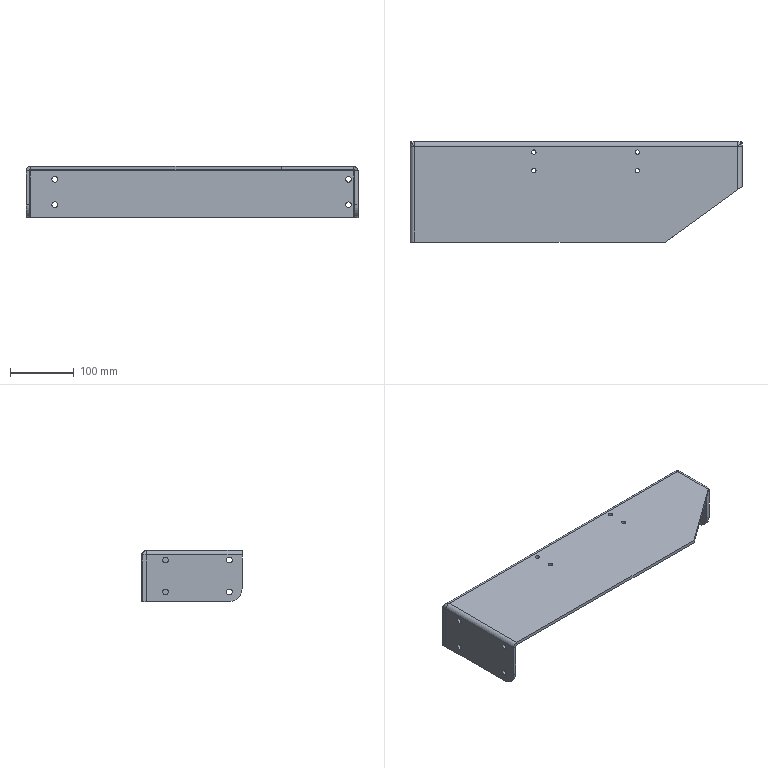Part | SolidWorks | features ICE 2, SMWeldBead 2, Cut 1, EdgeFlange 1, Fillet 1, FlatPattern 1, HoleWzd 1, SMBaseFlange 1, SheetMetal 1 | 1 solid | 71 faces | box 520 x 157 x 80 mm | volume 647127 mm3 | cylinder 42 | plane 26 | spline 3 | commonest cylinder face diameters 9 x14 6.8 x8 4 x7 14 x7 2 x2 8.927 x2